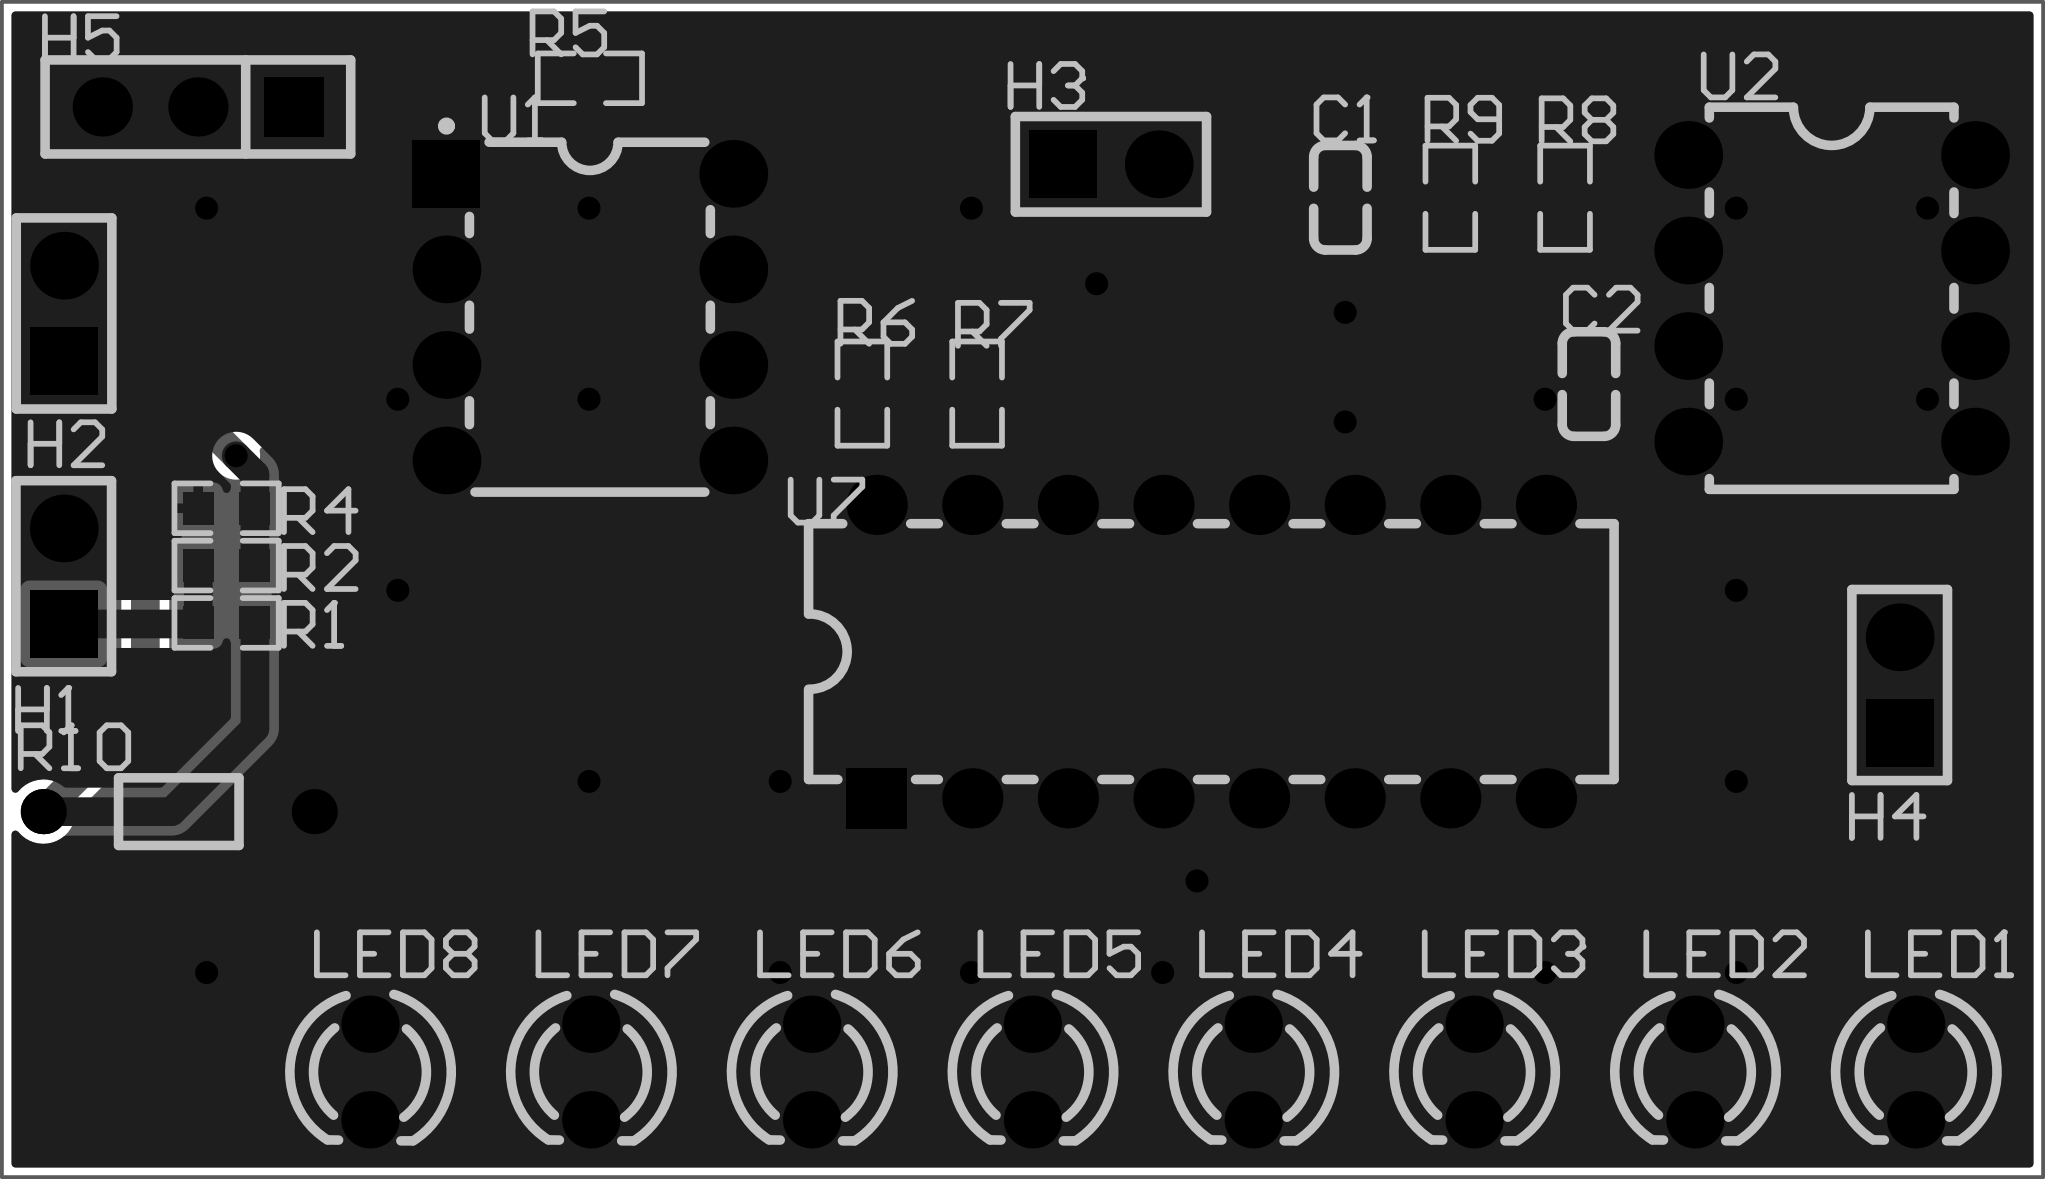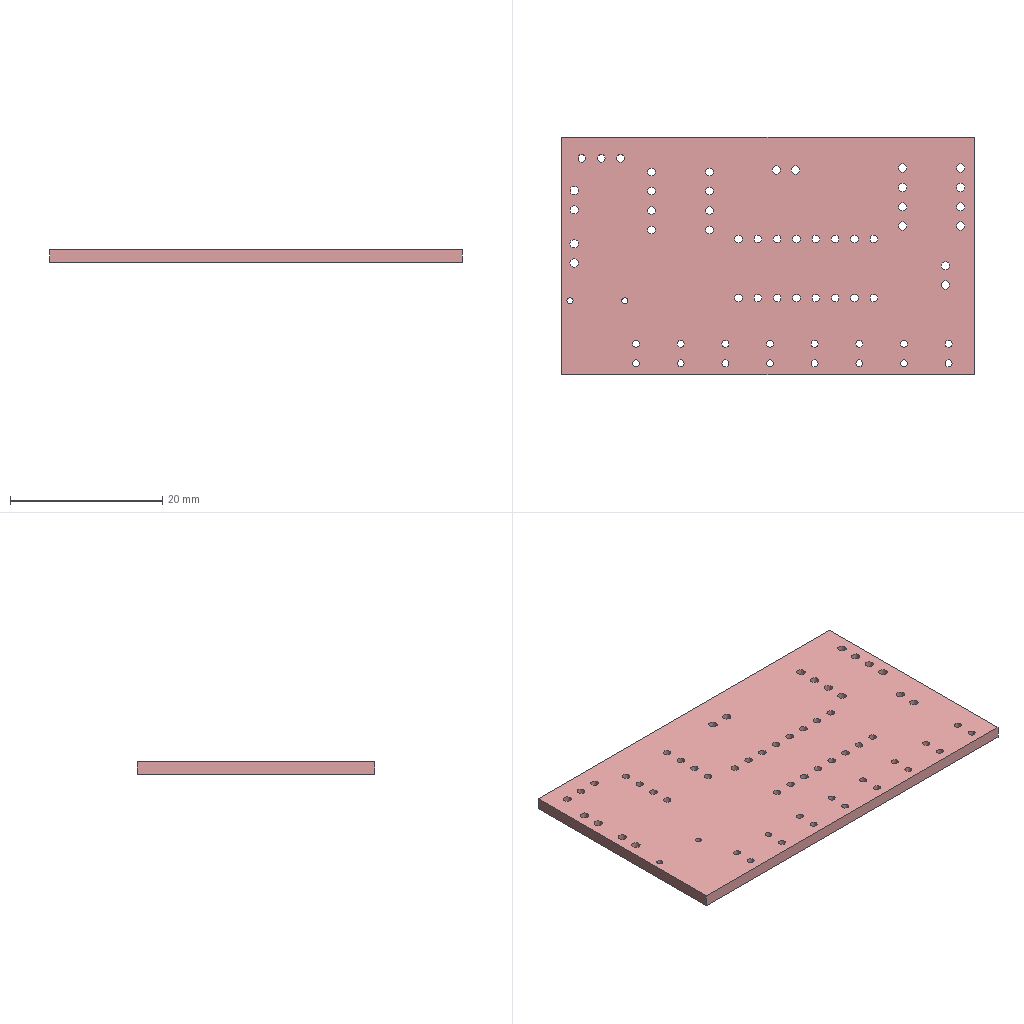Circuit board layout | Altium Designer | box 54.2 x 31.2 x 1.6 mm
Layer stack:
# Altium Designer layer stack of  (unit mm; dielectric type: 0 none, 1 core, 2 prepreg, 3 surface material)
index,name,kind,layer,copper_thickness_mm,dielectric_type,dielectric_thickness_mm,dielectric_material,dielectric_constant
0,Top Paste Mask Layer,other,,,,,,
1,Top Silkscreen Layer,other,,,,,,
2,Top Solder Mask Layer,dielectric,,,3,0.01,,3.3
3,Top Layer,copper,Top Layer,0.035,,,,
4,Dielectric1,dielectric,,,3,1.51,FR4,4.5
5,Bottom Layer,copper,Bottom Layer,0.035,,,,
6,Bottom Solder Mask Layer,dielectric,,,3,0.01,,3.3
7,Bottom Silkscreen Layer,other,,,,,,
8,Bottom Paste Mask Layer,other,,,,,,
# drill layer pairs: low layer,high layer
drill_pair,Top Layer,Bottom Layer
Part placement:
Designator,Comment,Layer,Footprint,Center-X(mm),Center-Y(mm),Rotation
C1,1.6uF,TopLayer,C0603,119.253,108.331,90
C2,1.6uF,TopLayer,C0603,125.857,103.378,90
H1,,TopLayer,HDR-TH_2P-P2.54-V-M-1,85.336,98.27,90
H2,,TopLayer,HDR-TH_2P-P2.54-V-M-1,85.344,105.255,90
H3,,TopLayer,HDR-TH_2P-P2.54-V-M-1,113.157,109.22,0
H4,,TopLayer,HDR-TH_2P-P2.54-V-M-1,134.112,95.377,90
LED1,,TopLayer,LED_TH-3mm,134.538,85.09,270
LED2,,TopLayer,LED_TH-3mm,128.671,85.09,270
LED3,,TopLayer,LED_TH-3mm,122.805,85.09,270
LED4,,TopLayer,LED_TH-3mm,116.938,85.09,270
LED5,,TopLayer,LED_TH-3mm,111.072,85.09,270
LED6,,TopLayer,LED_TH-3mm,105.205,85.09,270
LED7,,TopLayer,LED_TH-3mm,99.338,85.09,270
LED8,,TopLayer,LED_TH-3mm,93.472,85.09,270
R1,1K,TopLayer,R0603,89.662,97.028,0
R2,1K,TopLayer,R0603,89.662,98.552,0
R4,1K,TopLayer,R0603,89.662,100.076,180
R5,5.49kΩ,TopLayer,R0603,99.314,111.506,0
R8,10K,TopLayer,R0603,125.222,108.331,270
R9,10K,TopLayer,R0603,122.174,108.331,270
U1,AD620AN,TopLayer,DIP-8_L9.3-W6.4-P2.54-LS7.6-BL,99.314,105.156,270
U2,741,TopLayer,PDIP-8_L10.2-W6.5-P2.54-LS7.6-BL,132.304,105.658,270
U7,CD40175BF3A,TopLayer,CDIP-16_L21.4-W6.8-P2.54-LS7.8-BL,115.824,96.266,0
R6,1.5K,TopLayer,R0603,106.553,103.124,90
R7,1.5K,TopLayer,R0603,109.601,103.124,270
H5,,TopLayer,HDR-TH_3P-P2.54-V-F,88.9,110.744,180
R10,10kΩ,TopLayer,Res_1/8W,88.392,92.011,0
Pad and via stacks:
# Altium Designer via and pad stacks of  (unit mm). Each distinct definition once, with the count of objects using it.
# via: kind,start_layer,end_layer,hole_mm,diameter_mm,mode(0 simple;1 top-mid-bottom;2 full stack),diameter_per_layer,count,example_net
# pad: kind,layer,hole_mm,hole_type(0 round;1 square;2 slot),plating,top_size,top_shape(1 round;2 rect;3 octagon;9 rounded rect),mid_size,bottom_size,mode,footprint,size_per_layer,count,example
pad,Top Layer,0,0,plated,0.8x0.9,2,0.8x0.9,0.8x0.9,0,C0603,,4,C1.2
pad,Top Layer,0,0,plated,0.8065x0.864,2,0.8065x0.864,0.8065x0.864,0,R0603,,16,R1.2
pad,Multi-Layer,1.1,0,plated,1.8x1.8,1,1.8x1.8,1.8x1.8,0,HDR-TH_2P-P2.54-V-M-1,,4,H1.2
pad,Multi-Layer,1.1,0,plated,1.8x1.8,2,1.8x1.8,1.8x1.8,0,HDR-TH_2P-P2.54-V-M-1,,4,H1.1
pad,Multi-Layer,0.9144,0,plated,1.524x1.524,1,1.524x1.524,1.524x1.524,0,LED_TH-3mm,,16,LED1.1
pad,Multi-Layer,1,0,plated,1.8x1.8,2,1.8x1.8,1.8x1.8,0,DIP-8_L9.3-W6.4-P2.54-LS7.6-BL,,1,U1.1
pad,Multi-Layer,1,0,plated,1.8x1.8,1,1.8x1.8,1.8x1.8,0,DIP-8_L9.3-W6.4-P2.54-LS7.6-BL,,7,U1.2
pad,Multi-Layer,1.1,0,plated,1.8x1.8,1,1.8x1.8,1.8x1.8,0,PDIP-8_L10.2-W6.5-P2.54-LS7.6-BL,,8,U2.1
pad,Multi-Layer,1,0,plated,1.6x1.6,1,1.6x1.6,1.6x1.6,0,CDIP-16_L21.4-W6.8-P2.54-LS7.8-BL,,15,U7.16
pad,Multi-Layer,1,0,plated,1.6x1.6,2,1.6x1.6,1.6x1.6,0,CDIP-16_L21.4-W6.8-P2.54-LS7.8-BL,,1,U7.1
pad,Multi-Layer,1.02,0,plated,1.575x1.575,1,1.575x1.575,1.575x1.575,0,HDR-TH_3P-P2.54-V-F,,2,H5.3
pad,Multi-Layer,1.02,0,plated,1.575x1.575,2,1.575x1.575,1.575x1.575,0,HDR-TH_3P-P2.54-V-F,,1,H5.1
pad,Multi-Layer,0.8001,0,plated,1.199x1.199,1,1.199x1.199,1.199x1.199,0,Res_1/8W,,2,R10.1
via,Top Layer,Bottom Layer,0.3048,0.61,0,,26,$1N46
Copper pours:
name,layer,net,type(0 solid;1 hatched;2 none)
Bottom Layer-GND,Bottom Layer,GND,0
Top Layer-GND,Top Layer,GND,0